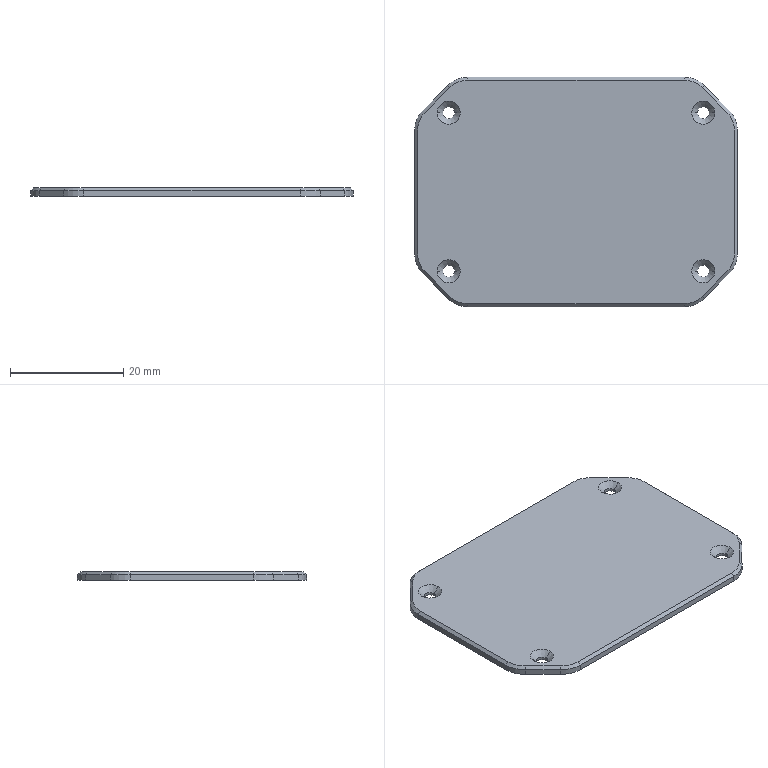NC program | NX | posted with a generic post | part box 57 x 40.5 x 1.5 mm
Lines 2968 to 4443 of 7802:
(PLANAR_PROFILE_COPY_3_COPY , TOOL : D4)
N5796 T01 M6
N5798 G54
N5800 G17 G0 G90 X-183.9 Y91.609 S6500 M3
N5802 G43 Z20. H1
N5804 Z0.1
N5806 G94 G1 Y68.668 Z0.06 F1200.
N5808 X-184.173 Y67.266 Z0.057
N5810 X-184.719 Y65.947 Z0.055
N5812 X-185.518 Y64.763 Z0.052
N5814 X-190.763 Y59.518 Z0.04
N5816 X-191.947 Y58.719 Z0.037
N5818 X-193.266 Y58.173 Z0.035
N5820 X-194.668 Y57.9 Z0.032
N5822 X-234.332 Z-0.037
N5824 X-235.734 Y58.173 Z-0.04
N5826 X-237.053 Y58.719 Z-0.042
N5828 X-238.237 Y59.518 Z-0.045
N5830 X-243.482 Y64.763 Z-0.058
N5832 X-244.281 Y65.947 Z-0.06
N5834 X-244.827 Y67.266 Z-0.063
N5836 X-245.1 Y68.668 Z-0.065
N5838 Y91.832 Z-0.106
N5840 X-244.827 Y93.234 Z-0.108
N5842 X-244.281 Y94.553 Z-0.11
N5844 X-243.482 Y95.737 Z-0.113
N5846 X-238.237 Y100.982 Z-0.126
N5848 X-237.053 Y101.781 Z-0.128
N5850 X-235.734 Y102.327 Z-0.131
N5852 X-234.332 Y102.6 Z-0.133
N5854 X-194.668 Z-0.203
N5856 X-193.266 Y102.327 Z-0.205
N5858 X-191.947 Y101.781 Z-0.208
N5860 X-190.763 Y100.982 Z-0.21
N5862 X-185.518 Y95.737 Z-0.223
N5864 X-184.719 Y94.553 Z-0.226
N5866 X-184.173 Y93.234 Z-0.228
N5868 X-183.9 Y91.832 Z-0.231
N5870 Y68.668 Z-0.271
N5872 X-184.173 Y67.266 Z-0.273
N5874 X-184.719 Y65.947 Z-0.276
N5876 X-185.518 Y64.763 Z-0.278
N5878 X-190.763 Y59.518 Z-0.291
N5880 X-191.947 Y58.719 Z-0.294
N5882 X-193.266 Y58.173 Z-0.296
N5884 X-194.668 Y57.9 Z-0.299
N5886 X-195.321 Z-0.3
N5888 X-233.679 F2000.
N5890 G2 X-238.699 Y59.98 R7.1
N5892 G1 X-243.02 Y64.301
N5894 G2 X-245.1 Y69.321 R7.1
N5896 G1 Y91.179
N5898 G2 X-243.02 Y96.199 R7.1
N5900 G1 X-238.699 Y100.52
N5902 G2 X-233.679 Y102.6 R7.1
N5904 G1 X-195.321
N5906 G2 X-190.301 Y100.52 R7.1
N5908 G1 X-185.98 Y96.199
N5910 G2 X-183.9 Y91.179 R7.1
N5912 G1 Y69.321
N5914 G2 X-185.98 Y64.301 R7.1
N5916 G1 X-190.301 Y59.98
N5918 G2 X-195.321 Y57.9 R7.1
N5920 G1 Z-0.2
N5922 G0 Z20.
N5924 X-183.9 Y91.609
N5926 Z-0.2
N5928 G1 Y68.668 Z-0.24 F1200.
N5930 X-184.173 Y67.266 Z-0.243
N5932 X-184.719 Y65.947 Z-0.245
N5934 X-185.518 Y64.763 Z-0.248
N5936 X-190.763 Y59.518 Z-0.26
N5938 X-191.947 Y58.719 Z-0.263
N5940 X-193.266 Y58.173 Z-0.265
N5942 X-194.668 Y57.9 Z-0.268
N5944 X-234.332 Z-0.337
N5946 X-235.734 Y58.173 Z-0.34
N5948 X-237.053 Y58.719 Z-0.342
N5950 X-238.237 Y59.518 Z-0.345
N5952 X-243.482 Y64.763 Z-0.358
N5954 X-244.281 Y65.947 Z-0.36
N5956 X-244.827 Y67.266 Z-0.363
N5958 X-245.1 Y68.668 Z-0.365
N5960 Y91.832 Z-0.406
N5962 X-244.827 Y93.234 Z-0.408
N5964 X-244.281 Y94.553 Z-0.41
N5966 X-243.482 Y95.737 Z-0.413
N5968 X-238.237 Y100.982 Z-0.426
N5970 X-237.053 Y101.781 Z-0.428
N5972 X-235.734 Y102.327 Z-0.431
N5974 X-234.332 Y102.6 Z-0.433
N5976 X-194.668 Z-0.503
N5978 X-193.266 Y102.327 Z-0.505
N5980 X-191.947 Y101.781 Z-0.508
N5982 X-190.763 Y100.982 Z-0.51
N5984 X-185.518 Y95.737 Z-0.523
N5986 X-184.719 Y94.553 Z-0.526
N5988 X-184.173 Y93.234 Z-0.528
N5990 X-183.9 Y91.832 Z-0.531
N5992 Y68.668 Z-0.571
N5994 X-184.173 Y67.266 Z-0.573
N5996 X-184.719 Y65.947 Z-0.576
N5998 X-185.518 Y64.763 Z-0.578
N6000 X-190.763 Y59.518 Z-0.591
N6002 X-191.947 Y58.719 Z-0.594
N6004 X-193.266 Y58.173 Z-0.596
N6006 X-194.668 Y57.9 Z-0.599
N6008 X-195.321 Z-0.6
N6010 X-233.679 F2000.
N6012 G2 X-238.699 Y59.98 R7.1
N6014 G1 X-243.02 Y64.301
N6016 G2 X-245.1 Y69.321 R7.1
N6018 G1 Y91.179
N6020 G2 X-243.02 Y96.199 R7.1
N6022 G1 X-238.699 Y100.52
N6024 G2 X-233.679 Y102.6 R7.1
N6026 G1 X-195.321
N6028 G2 X-190.301 Y100.52 R7.1
N6030 G1 X-185.98 Y96.199
N6032 G2 X-183.9 Y91.179 R7.1
N6034 G1 Y69.321
N6036 G2 X-185.98 Y64.301 R7.1
N6038 G1 X-190.301 Y59.98
N6040 G2 X-195.321 Y57.9 R7.1
N6042 G1 Z-0.5
N6044 G0 Z20.
N6046 X-183.9 Y91.609
N6048 Z-0.5
N6050 G1 Y68.668 Z-0.54 F1200.
N6052 X-184.173 Y67.266 Z-0.543
N6054 X-184.719 Y65.947 Z-0.545
N6056 X-185.518 Y64.763 Z-0.548
N6058 X-190.763 Y59.518 Z-0.56
N6060 X-191.947 Y58.719 Z-0.563
N6062 X-193.266 Y58.173 Z-0.565
N6064 X-194.668 Y57.9 Z-0.568
N6066 X-234.332 Z-0.637
N6068 X-235.734 Y58.173 Z-0.64
N6070 X-237.053 Y58.719 Z-0.642
N6072 X-238.237 Y59.518 Z-0.645
N6074 X-243.482 Y64.763 Z-0.658
N6076 X-244.281 Y65.947 Z-0.66
N6078 X-244.827 Y67.266 Z-0.663
N6080 X-245.1 Y68.668 Z-0.665
N6082 Y91.832 Z-0.706
N6084 X-244.827 Y93.234 Z-0.708
N6086 X-244.281 Y94.553 Z-0.71
N6088 X-243.482 Y95.737 Z-0.713
N6090 X-238.237 Y100.982 Z-0.726
N6092 X-237.053 Y101.781 Z-0.728
N6094 X-235.734 Y102.327 Z-0.731
N6096 X-234.332 Y102.6 Z-0.733
N6098 X-194.668 Z-0.803
N6100 X-193.266 Y102.327 Z-0.805
N6102 X-191.947 Y101.781 Z-0.808
N6104 X-190.763 Y100.982 Z-0.81
N6106 X-185.518 Y95.737 Z-0.823
N6108 X-184.719 Y94.553 Z-0.826
N6110 X-184.173 Y93.234 Z-0.828
N6112 X-183.9 Y91.832 Z-0.831
N6114 Y68.668 Z-0.871
N6116 X-184.173 Y67.266 Z-0.873
N6118 X-184.719 Y65.947 Z-0.876
N6120 X-185.518 Y64.763 Z-0.878
N6122 X-190.763 Y59.518 Z-0.891
N6124 X-191.947 Y58.719 Z-0.894
N6126 X-193.266 Y58.173 Z-0.896
N6128 X-194.668 Y57.9 Z-0.899
N6130 X-195.321 Z-0.9
N6132 X-233.679 F2000.
N6134 G2 X-238.699 Y59.98 R7.1
N6136 G1 X-243.02 Y64.301
N6138 G2 X-245.1 Y69.321 R7.1
N6140 G1 Y91.179
N6142 G2 X-243.02 Y96.199 R7.1
N6144 G1 X-238.699 Y100.52
N6146 G2 X-233.679 Y102.6 R7.1
N6148 G1 X-195.321
N6150 G2 X-190.301 Y100.52 R7.1
N6152 G1 X-185.98 Y96.199
N6154 G2 X-183.9 Y91.179 R7.1
N6156 G1 Y69.321
N6158 G2 X-185.98 Y64.301 R7.1
N6160 G1 X-190.301 Y59.98
N6162 G2 X-195.321 Y57.9 R7.1
N6164 G1 Z-0.8
N6166 G0 Z20.
N6168 X-183.9 Y91.609
N6170 Z-0.8
N6172 G1 Y68.668 Z-0.84 F1200.
N6174 X-184.173 Y67.266 Z-0.843
N6176 X-184.719 Y65.947 Z-0.845
N6178 X-185.518 Y64.763 Z-0.848
N6180 X-190.763 Y59.518 Z-0.86
N6182 X-191.947 Y58.719 Z-0.863
N6184 X-193.266 Y58.173 Z-0.865
N6186 X-194.668 Y57.9 Z-0.868
N6188 X-234.332 Z-0.937
N6190 X-235.734 Y58.173 Z-0.94
N6192 X-237.053 Y58.719 Z-0.942
N6194 X-238.237 Y59.518 Z-0.945
N6196 X-243.482 Y64.763 Z-0.958
N6198 X-244.281 Y65.947 Z-0.96
N6200 X-244.827 Y67.266 Z-0.963
N6202 X-245.1 Y68.668 Z-0.965
N6204 Y91.832 Z-1.006
N6206 X-244.827 Y93.234 Z-1.008
N6208 X-244.281 Y94.553 Z-1.01
N6210 X-243.482 Y95.737 Z-1.013
N6212 X-238.237 Y100.982 Z-1.026
N6214 X-237.053 Y101.781 Z-1.028
N6216 X-235.734 Y102.327 Z-1.031
N6218 X-234.332 Y102.6 Z-1.033
N6220 X-194.668 Z-1.103
N6222 X-193.266 Y102.327 Z-1.105
N6224 X-191.947 Y101.781 Z-1.108
N6226 X-190.763 Y100.982 Z-1.11
N6228 X-185.518 Y95.737 Z-1.123
N6230 X-184.719 Y94.553 Z-1.126
N6232 X-184.173 Y93.234 Z-1.128
N6234 X-183.9 Y91.832 Z-1.131
N6236 Y68.668 Z-1.171
N6238 X-184.173 Y67.266 Z-1.173
N6240 X-184.719 Y65.947 Z-1.176
N6242 X-185.518 Y64.763 Z-1.178
N6244 X-190.763 Y59.518 Z-1.191
N6246 X-191.947 Y58.719 Z-1.194
N6248 X-193.266 Y58.173 Z-1.196
N6250 X-194.668 Y57.9 Z-1.199
N6252 X-195.321 Z-1.2
N6254 X-233.679 F2000.
N6256 G2 X-238.699 Y59.98 R7.1
N6258 G1 X-243.02 Y64.301
N6260 G2 X-245.1 Y69.321 R7.1
N6262 G1 Y91.179
N6264 G2 X-243.02 Y96.199 R7.1
N6266 G1 X-238.699 Y100.52
N6268 G2 X-233.679 Y102.6 R7.1
N6270 G1 X-195.321
N6272 G2 X-190.301 Y100.52 R7.1
N6274 G1 X-185.98 Y96.199
N6276 G2 X-183.9 Y91.179 R7.1
N6278 G1 Y69.321
N6280 G2 X-185.98 Y64.301 R7.1
N6282 G1 X-190.301 Y59.98
N6284 G2 X-195.321 Y57.9 R7.1
N6286 G1 Z-1.1
N6288 G0 Z20.
N6290 X-183.9 Y91.609
N6292 Z-1.1
N6294 G1 Y68.668 Z-1.14 F1200.
N6296 X-184.173 Y67.266 Z-1.143
N6298 X-184.719 Y65.947 Z-1.145
N6300 X-185.518 Y64.763 Z-1.148
N6302 X-190.763 Y59.518 Z-1.16
N6304 X-191.947 Y58.719 Z-1.163
N6306 X-193.266 Y58.173 Z-1.165
N6308 X-194.668 Y57.9 Z-1.168
N6310 X-234.332 Z-1.237
N6312 X-235.734 Y58.173 Z-1.24
N6314 X-237.053 Y58.719 Z-1.242
N6316 X-238.237 Y59.518 Z-1.245
N6318 X-243.482 Y64.763 Z-1.258
N6320 X-244.281 Y65.947 Z-1.26
N6322 X-244.827 Y67.266 Z-1.263
N6324 X-245.1 Y68.668 Z-1.265
N6326 Y91.832 Z-1.306
N6328 X-244.827 Y93.234 Z-1.308
N6330 X-244.281 Y94.553 Z-1.31
N6332 X-243.482 Y95.737 Z-1.313
N6334 X-238.237 Y100.982 Z-1.326
N6336 X-237.053 Y101.781 Z-1.328
N6338 X-235.734 Y102.327 Z-1.331
N6340 X-234.332 Y102.6 Z-1.333
N6342 X-194.668 Z-1.403
N6344 X-193.266 Y102.327 Z-1.405
N6346 X-191.947 Y101.781 Z-1.408
N6348 X-190.763 Y100.982 Z-1.41
N6350 X-185.518 Y95.737 Z-1.423
N6352 X-184.719 Y94.553 Z-1.426
N6354 X-184.173 Y93.234 Z-1.428
N6356 X-183.9 Y91.832 Z-1.431
N6358 Y68.668 Z-1.471
N6360 X-184.173 Y67.266 Z-1.473
N6362 X-184.719 Y65.947 Z-1.476
N6364 X-185.518 Y64.763 Z-1.478
N6366 X-190.763 Y59.518 Z-1.491
N6368 X-191.947 Y58.719 Z-1.494
N6370 X-193.266 Y58.173 Z-1.496
N6372 X-194.668 Y57.9 Z-1.499
N6374 X-195.321 Z-1.5
N6376 X-233.679 F2000.
N6378 G2 X-238.699 Y59.98 R7.1
N6380 G1 X-243.02 Y64.301
N6382 G2 X-245.1 Y69.321 R7.1
N6384 G1 Y91.179
N6386 G2 X-243.02 Y96.199 R7.1
N6388 G1 X-238.699 Y100.52
N6390 G2 X-233.679 Y102.6 R7.1
N6392 G1 X-195.321
N6394 G2 X-190.301 Y100.52 R7.1
N6396 G1 X-185.98 Y96.199
N6398 G2 X-183.9 Y91.179 R7.1
N6400 G1 Y69.321
N6402 G2 X-185.98 Y64.301 R7.1
N6404 G1 X-190.301 Y59.98
N6406 G2 X-195.321 Y57.9 R7.1
N6408 G1 Z-1.4
N6410 G0 Z20.
(PLANAR_PROFILE_COPY_COPY_3_COPY , TOOL : D4)
N6412 X-195.221
N6414 Z1.5
N6416 G1 Z-1.5 F800.
N6418 X-195.232 Y57.952
N6420 X-195.27 Y57.989
N6422 X-195.321 Y58.
N6424 X-233.679
N6426 G2 X-238.629 Y60.05 R7.
N6428 G1 X-242.95 Y64.371
N6430 G2 X-245. Y69.321 R7.
N6432 G1 Y91.179
N6434 G2 X-242.95 Y96.129 R7.
N6436 G1 X-238.629 Y100.45
N6438 G2 X-233.679 Y102.5 R7.
N6440 G1 X-195.321
N6442 G2 X-190.371 Y100.45 R7.
N6444 G1 X-186.05 Y96.129
N6446 G2 X-184. Y91.179 R7.
N6448 G1 Y69.321
N6450 G2 X-186.05 Y64.371 R7.
N6452 G1 X-190.371 Y60.05
N6454 G2 X-195.321 Y58. R7.
N6456 G1 X-195.373 Y57.989
N6458 X-195.41 Y57.952
N6460 X-195.421 Y57.9
N6462 Z1.5
N6464 G0 Z20.
N6466 M5
(PLANAR_PROFILE_COPY_COPY_COPY_2_COPY , TOOL : D3倒角)
N6468 T02 M6
N6470 G54
N6472 G17 G0 G90 X-193.321 Y57.4 S4500 M3
N6474 G43 Z20. H2
N6476 Z2.
N6478 G94 G1 Z-1. F800.
N6480 G3 X-195.321 Y59.4 R2.
N6482 G1 X-233.679
N6484 G2 X-237.639 Y61.04 R5.6
N6486 G1 X-241.96 Y65.361
N6488 G2 X-243.6 Y69.321 R5.6
N6490 G1 Y91.179
N6492 G2 X-241.96 Y95.139 R5.6
N6494 G1 X-237.639 Y99.46
N6496 G2 X-233.679 Y101.1 R5.6
N6498 G1 X-195.321
N6500 G2 X-191.361 Y99.46 R5.6
N6502 G1 X-187.04 Y95.139
N6504 G2 X-185.4 Y91.179 R5.6
N6506 G1 Y69.321
N6508 G2 X-187.04 Y65.361 R5.6
N6510 G1 X-191.361 Y61.04
N6512 G2 X-195.321 Y59.4 R5.6
N6514 G3 X-197.321 Y57.4 R2.
N6516 G1 Z2.
N6518 G0 Z20.
N6520 M5
(PLANAR_PROFILE_COPY_4_COPY , TOOL : D4)
N6522 T01 M6
N6524 G54
N6526 G17 G0 G90 X-245.9 Y91.609 S6500 M3
N6528 G43 Z20. H1
N6530 Z0.1
N6532 G94 G1 Y68.668 Z0.06 F1200.
N6534 X-246.173 Y67.266 Z0.057
N6536 X-246.719 Y65.947 Z0.055
N6538 X-247.518 Y64.763 Z0.052
N6540 X-252.763 Y59.518 Z0.04
N6542 X-253.947 Y58.719 Z0.037
N6544 X-255.266 Y58.173 Z0.035
N6546 X-256.668 Y57.9 Z0.032
N6548 X-296.332 Z-0.037
N6550 X-297.734 Y58.173 Z-0.04
N6552 X-299.053 Y58.719 Z-0.042
N6554 X-300.237 Y59.518 Z-0.045
N6556 X-305.482 Y64.763 Z-0.058
N6558 X-306.281 Y65.947 Z-0.06
N6560 X-306.827 Y67.266 Z-0.063
N6562 X-307.1 Y68.668 Z-0.065
N6564 Y91.832 Z-0.106
N6566 X-306.827 Y93.234 Z-0.108
N6568 X-306.281 Y94.553 Z-0.11
N6570 X-305.482 Y95.737 Z-0.113
N6572 X-300.237 Y100.982 Z-0.126
N6574 X-299.053 Y101.781 Z-0.128
N6576 X-297.734 Y102.327 Z-0.131
N6578 X-296.332 Y102.6 Z-0.133
N6580 X-256.668 Z-0.203
N6582 X-255.266 Y102.327 Z-0.205
N6584 X-253.947 Y101.781 Z-0.208
N6586 X-252.763 Y100.982 Z-0.21
N6588 X-247.518 Y95.737 Z-0.223
N6590 X-246.719 Y94.553 Z-0.226
N6592 X-246.173 Y93.234 Z-0.228
N6594 X-245.9 Y91.832 Z-0.231
N6596 Y68.668 Z-0.271
N6598 X-246.173 Y67.266 Z-0.273
N6600 X-246.719 Y65.947 Z-0.276
N6602 X-247.518 Y64.763 Z-0.278
N6604 X-252.763 Y59.518 Z-0.291
N6606 X-253.947 Y58.719 Z-0.294
N6608 X-255.266 Y58.173 Z-0.296
N6610 X-256.668 Y57.9 Z-0.299
N6612 X-257.321 Z-0.3
N6614 X-295.679 F2000.
N6616 G2 X-300.699 Y59.98 R7.1
N6618 G1 X-305.02 Y64.301
N6620 G2 X-307.1 Y69.321 R7.1
N6622 G1 Y91.179
N6624 G2 X-305.02 Y96.199 R7.1
N6626 G1 X-300.699 Y100.52
N6628 G2 X-295.679 Y102.6 R7.1
N6630 G1 X-257.321
N6632 G2 X-252.301 Y100.52 R7.1
N6634 G1 X-247.98 Y96.199
N6636 G2 X-245.9 Y91.179 R7.1
N6638 G1 Y69.321
N6640 G2 X-247.98 Y64.301 R7.1
N6642 G1 X-252.301 Y59.98
N6644 G2 X-257.321 Y57.9 R7.1
N6646 G1 Z-0.2
N6648 G0 Z20.
N6650 X-245.9 Y91.609
N6652 Z-0.2
N6654 G1 Y68.668 Z-0.24 F1200.
N6656 X-246.173 Y67.266 Z-0.243
N6658 X-246.719 Y65.947 Z-0.245
N6660 X-247.518 Y64.763 Z-0.248
N6662 X-252.763 Y59.518 Z-0.26
N6664 X-253.947 Y58.719 Z-0.263
N6666 X-255.266 Y58.173 Z-0.265
N6668 X-256.668 Y57.9 Z-0.268
N6670 X-296.332 Z-0.337
N6672 X-297.734 Y58.173 Z-0.34
N6674 X-299.053 Y58.719 Z-0.342
N6676 X-300.237 Y59.518 Z-0.345
N6678 X-305.482 Y64.763 Z-0.358
N6680 X-306.281 Y65.947 Z-0.36
N6682 X-306.827 Y67.266 Z-0.363
N6684 X-307.1 Y68.668 Z-0.365
N6686 Y91.832 Z-0.406
N6688 X-306.827 Y93.234 Z-0.408
N6690 X-306.281 Y94.553 Z-0.41
N6692 X-305.482 Y95.737 Z-0.413
N6694 X-300.237 Y100.982 Z-0.426
N6696 X-299.053 Y101.781 Z-0.428
N6698 X-297.734 Y102.327 Z-0.431
N6700 X-296.332 Y102.6 Z-0.433
N6702 X-256.668 Z-0.503
N6704 X-255.266 Y102.327 Z-0.505
N6706 X-253.947 Y101.781 Z-0.508
N6708 X-252.763 Y100.982 Z-0.51
N6710 X-247.518 Y95.737 Z-0.523
N6712 X-246.719 Y94.553 Z-0.526
N6714 X-246.173 Y93.234 Z-0.528
N6716 X-245.9 Y91.832 Z-0.531
N6718 Y68.668 Z-0.571
N6720 X-246.173 Y67.266 Z-0.573
N6722 X-246.719 Y65.947 Z-0.576
N6724 X-247.518 Y64.763 Z-0.578
N6726 X-252.763 Y59.518 Z-0.591
N6728 X-253.947 Y58.719 Z-0.594
N6730 X-255.266 Y58.173 Z-0.596
N6732 X-256.668 Y57.9 Z-0.599
N6734 X-257.321 Z-0.6
N6736 X-295.679 F2000.
N6738 G2 X-300.699 Y59.98 R7.1
N6740 G1 X-305.02 Y64.301
N6742 G2 X-307.1 Y69.321 R7.1
N6744 G1 Y91.179
N6746 G2 X-305.02 Y96.199 R7.1
N6748 G1 X-300.699 Y100.52
N6750 G2 X-295.679 Y102.6 R7.1
N6752 G1 X-257.321
N6754 G2 X-252.301 Y100.52 R7.1
N6756 G1 X-247.98 Y96.199
N6758 G2 X-245.9 Y91.179 R7.1
N6760 G1 Y69.321
N6762 G2 X-247.98 Y64.301 R7.1
N6764 G1 X-252.301 Y59.98
N6766 G2 X-257.321 Y57.9 R7.1
N6768 G1 Z-0.5
N6770 G0 Z20.
N6772 X-245.9 Y91.609
N6774 Z-0.5
N6776 G1 Y68.668 Z-0.54 F1200.
N6778 X-246.173 Y67.266 Z-0.543
N6780 X-246.719 Y65.947 Z-0.545
N6782 X-247.518 Y64.763 Z-0.548
N6784 X-252.763 Y59.518 Z-0.56
N6786 X-253.947 Y58.719 Z-0.563
N6788 X-255.266 Y58.173 Z-0.565
N6790 X-256.668 Y57.9 Z-0.568
N6792 X-296.332 Z-0.637
N6794 X-297.734 Y58.173 Z-0.64
N6796 X-299.053 Y58.719 Z-0.642
N6798 X-300.237 Y59.518 Z-0.645
N6800 X-305.482 Y64.763 Z-0.658
N6802 X-306.281 Y65.947 Z-0.66
N6804 X-306.827 Y67.266 Z-0.663
N6806 X-307.1 Y68.668 Z-0.665
N6808 Y91.832 Z-0.706
N6810 X-306.827 Y93.234 Z-0.708
N6812 X-306.281 Y94.553 Z-0.71
N6814 X-305.482 Y95.737 Z-0.713
N6816 X-300.237 Y100.982 Z-0.726
N6818 X-299.053 Y101.781 Z-0.728
N6820 X-297.734 Y102.327 Z-0.731
N6822 X-296.332 Y102.6 Z-0.733
N6824 X-256.668 Z-0.803
N6826 X-255.266 Y102.327 Z-0.805
N6828 X-253.947 Y101.781 Z-0.808
N6830 X-252.763 Y100.982 Z-0.81
N6832 X-247.518 Y95.737 Z-0.823
N6834 X-246.719 Y94.553 Z-0.826
N6836 X-246.173 Y93.234 Z-0.828
N6838 X-245.9 Y91.832 Z-0.831
N6840 Y68.668 Z-0.871
N6842 X-246.173 Y67.266 Z-0.873
N6844 X-246.719 Y65.947 Z-0.876
N6846 X-247.518 Y64.763 Z-0.878
N6848 X-252.763 Y59.518 Z-0.891
N6850 X-253.947 Y58.719 Z-0.894
N6852 X-255.266 Y58.173 Z-0.896
N6854 X-256.668 Y57.9 Z-0.899
N6856 X-257.321 Z-0.9
N6858 X-295.679 F2000.
N6860 G2 X-300.699 Y59.98 R7.1
N6862 G1 X-305.02 Y64.301
N6864 G2 X-307.1 Y69.321 R7.1
N6866 G1 Y91.179
N6868 G2 X-305.02 Y96.199 R7.1
N6870 G1 X-300.699 Y100.52
N6872 G2 X-295.679 Y102.6 R7.1
N6874 G1 X-257.321
N6876 G2 X-252.301 Y100.52 R7.1
N6878 G1 X-247.98 Y96.199
N6880 G2 X-245.9 Y91.179 R7.1
N6882 G1 Y69.321
N6884 G2 X-247.98 Y64.301 R7.1
N6886 G1 X-252.301 Y59.98
N6888 G2 X-257.321 Y57.9 R7.1
N6890 G1 Z-0.8
N6892 G0 Z20.
N6894 X-245.9 Y91.609
N6896 Z-0.8
N6898 G1 Y68.668 Z-0.84 F1200.
N6900 X-246.173 Y67.266 Z-0.843
N6902 X-246.719 Y65.947 Z-0.845
N6904 X-247.518 Y64.763 Z-0.848
N6906 X-252.763 Y59.518 Z-0.86
N6908 X-253.947 Y58.719 Z-0.863
N6910 X-255.266 Y58.173 Z-0.865
N6912 X-256.668 Y57.9 Z-0.868
N6914 X-296.332 Z-0.937
N6916 X-297.734 Y58.173 Z-0.94
N6918 X-299.053 Y58.719 Z-0.942
N6920 X-300.237 Y59.518 Z-0.945
N6922 X-305.482 Y64.763 Z-0.958
N6924 X-306.281 Y65.947 Z-0.96
N6926 X-306.827 Y67.266 Z-0.963
N6928 X-307.1 Y68.668 Z-0.965
N6930 Y91.832 Z-1.006
N6932 X-306.827 Y93.234 Z-1.008
N6934 X-306.281 Y94.553 Z-1.01
N6936 X-305.482 Y95.737 Z-1.013
N6938 X-300.237 Y100.982 Z-1.026
N6940 X-299.053 Y101.781 Z-1.028
N6942 X-297.734 Y102.327 Z-1.031
N6944 X-296.332 Y102.6 Z-1.033
N6946 X-256.668 Z-1.103
N6948 X-255.266 Y102.327 Z-1.105
N6950 X-253.947 Y101.781 Z-1.108
N6952 X-252.763 Y100.982 Z-1.11
N6954 X-247.518 Y95.737 Z-1.123
N6956 X-246.719 Y94.553 Z-1.126
N6958 X-246.173 Y93.234 Z-1.128
N6960 X-245.9 Y91.832 Z-1.131
N6962 Y68.668 Z-1.171
N6964 X-246.173 Y67.266 Z-1.173
N6966 X-246.719 Y65.947 Z-1.176
N6968 X-247.518 Y64.763 Z-1.178
N6970 X-252.763 Y59.518 Z-1.191
N6972 X-253.947 Y58.719 Z-1.194
N6974 X-255.266 Y58.173 Z-1.196
N6976 X-256.668 Y57.9 Z-1.199
N6978 X-257.321 Z-1.2
N6980 X-295.679 F2000.
N6982 G2 X-300.699 Y59.98 R7.1
N6984 G1 X-305.02 Y64.301
N6986 G2 X-307.1 Y69.321 R7.1
N6988 G1 Y91.179
N6990 G2 X-305.02 Y96.199 R7.1
N6992 G1 X-300.699 Y100.52
N6994 G2 X-295.679 Y102.6 R7.1
N6996 G1 X-257.321
N6998 G2 X-252.301 Y100.52 R7.1
N7000 G1 X-247.98 Y96.199
N7002 G2 X-245.9 Y91.179 R7.1
N7004 G1 Y69.321
N7006 G2 X-247.98 Y64.301 R7.1
N7008 G1 X-252.301 Y59.98
N7010 G2 X-257.321 Y57.9 R7.1
N7012 G1 Z-1.1
N7014 G0 Z20.
N7016 X-302.406 Y61.686
N7018 Z-1.1
N7020 G1 X-305.482 Y64.763 Z-1.108 F1200.
N7022 X-306.281 Y65.947 Z-1.11
N7024 X-306.827 Y67.266 Z-1.113
N7026 X-307.1 Y68.668 Z-1.115
N7028 Y91.832 Z-1.156
N7030 X-306.827 Y93.234 Z-1.158
N7032 X-306.281 Y94.553 Z-1.16
N7034 X-305.482 Y95.737 Z-1.163
N7036 X-300.237 Y100.982 Z-1.176
N7038 X-299.053 Y101.781 Z-1.178
N7040 X-297.734 Y102.327 Z-1.181
N7042 X-296.332 Y102.6 Z-1.183
N7044 X-256.668 Z-1.253
N7046 X-255.266 Y102.327 Z-1.255
N7048 X-253.947 Y101.781 Z-1.258
N7050 X-252.763 Y100.982 Z-1.26
N7052 X-247.518 Y95.737 Z-1.273
N7054 X-246.719 Y94.553 Z-1.276
N7056 X-246.173 Y93.234 Z-1.278
N7058 X-245.9 Y91.832 Z-1.281
N7060 Y68.668 Z-1.321
N7062 X-246.173 Y67.266 Z-1.323
N7064 X-246.719 Y65.947 Z-1.326
N7066 X-247.518 Y64.763 Z-1.328
N7068 X-252.763 Y59.518 Z-1.341
N7070 X-253.947 Y58.719 Z-1.344
N7072 X-255.266 Y58.173 Z-1.346
N7074 X-256.668 Y57.9 Z-1.349
N7076 X-257.321 Z-1.35
N7078 X-295.679 F2000.
N7080 G2 X-300.699 Y59.98 R7.1
N7082 G1 X-305.02 Y64.301
N7084 G2 X-307.1 Y69.321 R7.1
N7086 G1 Y91.179
N7088 G2 X-305.02 Y96.199 R7.1
N7090 G1 X-300.699 Y100.52
N7092 G2 X-295.679 Y102.6 R7.1
N7094 G1 X-257.321
N7096 G2 X-252.301 Y100.52 R7.1
N7098 G1 X-247.98 Y96.199
N7100 G2 X-245.9 Y91.179 R7.1
N7102 G1 Y69.321
N7104 G2 X-247.98 Y64.301 R7.1
N7106 G1 X-252.301 Y59.98
N7108 G2 X-257.321 Y57.9 R7.1
N7110 G1 Z-1.25
N7112 G0 Z20.
(PLANAR_PROFILE_COPY_COPY_4_COPY , TOOL : D4)
N7114 X-257.221
N7116 Z1.65
N7118 G1 Z-1.35 F800.
N7120 X-257.232 Y57.952
N7122 X-257.27 Y57.989
N7124 X-257.321 Y58.
N7126 X-295.679
N7128 G2 X-300.629 Y60.05 R7.
N7130 G1 X-304.95 Y64.371
N7132 G2 X-307. Y69.321 R7.
N7134 G1 Y91.179
N7136 G2 X-304.95 Y96.129 R7.
N7138 G1 X-300.629 Y100.45
N7140 G2 X-295.679 Y102.5 R7.
N7142 G1 X-257.321
N7144 G2 X-252.371 Y100.45 R7.
N7146 G1 X-248.05 Y96.129
N7148 G2 X-246. Y91.179 R7.
N7150 G1 Y69.321
N7152 G2 X-248.05 Y64.371 R7.
N7154 G1 X-252.371 Y60.05
N7156 G2 X-257.321 Y58. R7.
N7158 G1 X-257.373 Y57.989
N7160 X-257.41 Y57.952
N7162 X-257.421 Y57.9
N7164 Z1.65
N7166 G0 Z20.
N7168 M5
(PLANAR_PROFILE_COPY_COPY_COPY_3_COPY , TOOL : D3倒角)
N7170 T02 M6
N7172 G54
N7174 G17 G0 G90 X-255.321 Y57.4 S4500 M3
N7176 G43 Z20. H2
N7178 Z2.
N7180 G94 G1 Z-1. F800.
N7182 G3 X-257.321 Y59.4 R2.
N7184 G1 X-295.679
N7186 G2 X-299.639 Y61.04 R5.6
N7188 G1 X-303.96 Y65.361
N7190 G2 X-305.6 Y69.321 R5.6
N7192 G1 Y91.179
N7194 G2 X-303.96 Y95.139 R5.6
N7196 G1 X-299.639 Y99.46
N7198 G2 X-295.679 Y101.1 R5.6
N7200 G1 X-257.321
N7202 G2 X-253.361 Y99.46 R5.6
N7204 G1 X-249.04 Y95.139
N7206 G2 X-247.4 Y91.179 R5.6
N7208 G1 Y69.321
N7210 G2 X-249.04 Y65.361 R5.6
N7212 G1 X-253.361 Y61.04
N7214 G2 X-257.321 Y59.4 R5.6
N7216 G3 X-259.321 Y57.4 R2.
N7218 G1 Z2.
N7220 G0 Z20.
N7222 M5
(PLANAR_PROFILE_COPY_6 , TOOL : D4)
N7224 T01 M6
N7226 G54
N7228 G17 G0 G90 X2.1 Y151.609 S6500 M3
N7230 G43 Z20. H1
N7232 Z0.1
N7234 G94 G1 Y128.668 Z0.06 F1200.
N7236 X1.827 Y127.266 Z0.057
N7238 X1.281 Y125.947 Z0.055
N7240 X0.482 Y124.763 Z0.052
N7242 X-4.763 Y119.518 Z0.04
N7244 X-5.947 Y118.719 Z0.037
N7246 X-7.266 Y118.173 Z0.035
N7248 X-8.668 Y117.9 Z0.032
N7250 X-48.332 Z-0.037
N7252 X-49.734 Y118.173 Z-0.04
N7254 X-51.053 Y118.719 Z-0.042
N7256 X-52.237 Y119.518 Z-0.045
N7258 X-57.482 Y124.763 Z-0.058
N7260 X-58.281 Y125.947 Z-0.06
N7262 X-58.827 Y127.266 Z-0.063
N7264 X-59.1 Y128.668 Z-0.065
N7266 Y151.832 Z-0.106
N7268 X-58.827 Y153.234 Z-0.108
N7270 X-58.281 Y154.553 Z-0.11
N7272 X-57.482 Y155.737 Z-0.113
N7274 X-52.237 Y160.982 Z-0.126
N7276 X-51.053 Y161.781 Z-0.128
N7278 X-49.734 Y162.327 Z-0.131
N7280 X-48.332 Y162.6 Z-0.133
N7282 X-8.668 Z-0.203
N7284 X-7.266 Y162.327 Z-0.205
N7286 X-5.947 Y161.781 Z-0.208
N7288 X-4.763 Y160.982 Z-0.21
N7290 X0.482 Y155.737 Z-0.223
N7292 X1.281 Y154.553 Z-0.226
N7294 X1.827 Y153.234 Z-0.228
N7296 X2.1 Y151.832 Z-0.231
N7298 Y128.668 Z-0.271
N7300 X1.827 Y127.266 Z-0.273
N7302 X1.281 Y125.947 Z-0.276
N7304 X0.482 Y124.763 Z-0.278
N7306 X-4.763 Y119.518 Z-0.291
N7308 X-5.947 Y118.719 Z-0.294
N7310 X-7.266 Y118.173 Z-0.296
N7312 X-8.668 Y117.9 Z-0.299
N7314 X-9.321 Z-0.3
N7316 X-47.679 F2000.
N7318 G2 X-52.699 Y119.98 R7.1
N7320 G1 X-57.02 Y124.301
N7322 G2 X-59.1 Y129.321 R7.1
N7324 G1 Y151.179
N7326 G2 X-57.02 Y156.199 R7.1
N7328 G1 X-52.699 Y160.52
N7330 G2 X-47.679 Y162.6 R7.1
N7332 G1 X-9.321
N7334 G2 X-4.301 Y160.52 R7.1
N7336 G1 X0.02 Y156.199
N7338 G2 X2.1 Y151.179 R7.1
N7340 G1 Y129.321
N7342 G2 X0.02 Y124.301 R7.1
N7344 G1 X-4.301 Y119.98
N7346 G2 X-9.321 Y117.9 R7.1
N7348 G1 Z-0.2
N7350 G0 Z20.
N7352 X2.1 Y151.609
N7354 Z-0.2
N7356 G1 Y128.668 Z-0.24 F1200.
N7358 X1.827 Y127.266 Z-0.243
N7360 X1.281 Y125.947 Z-0.245
N7362 X0.482 Y124.763 Z-0.248
N7364 X-4.763 Y119.518 Z-0.26
N7366 X-5.947 Y118.719 Z-0.263
N7368 X-7.266 Y118.173 Z-0.265
N7370 X-8.668 Y117.9 Z-0.268
N7372 X-48.332 Z-0.337
N7374 X-49.734 Y118.173 Z-0.34
N7376 X-51.053 Y118.719 Z-0.342
N7378 X-52.237 Y119.518 Z-0.345
N7380 X-57.482 Y124.763 Z-0.358
N7382 X-58.281 Y125.947 Z-0.36
N7384 X-58.827 Y127.266 Z-0.363
N7386 X-59.1 Y128.668 Z-0.365
N7388 Y151.832 Z-0.406
N7390 X-58.827 Y153.234 Z-0.408
N7392 X-58.281 Y154.553 Z-0.41
N7394 X-57.482 Y155.737 Z-0.413
N7396 X-52.237 Y160.982 Z-0.426
N7398 X-51.053 Y161.781 Z-0.428
N7400 X-49.734 Y162.327 Z-0.431
N7402 X-48.332 Y162.6 Z-0.433
N7404 X-8.668 Z-0.503
N7406 X-7.266 Y162.327 Z-0.505
N7408 X-5.947 Y161.781 Z-0.508
N7410 X-4.763 Y160.982 Z-0.51
N7412 X0.482 Y155.737 Z-0.523
N7414 X1.281 Y154.553 Z-0.526
N7416 X1.827 Y153.234 Z-0.528
N7418 X2.1 Y151.832 Z-0.531
N7420 Y128.668 Z-0.571
N7422 X1.827 Y127.266 Z-0.573
N7424 X1.281 Y125.947 Z-0.576
N7426 X0.482 Y124.763 Z-0.578
N7428 X-4.763 Y119.518 Z-0.591
N7430 X-5.947 Y118.719 Z-0.594
N7432 X-7.266 Y118.173 Z-0.596
N7434 X-8.668 Y117.9 Z-0.599
N7436 X-9.321 Z-0.6
N7438 X-47.679 F2000.
N7440 G2 X-52.699 Y119.98 R7.1
N7442 G1 X-57.02 Y124.301
N7444 G2 X-59.1 Y129.321 R7.1
N7446 G1 Y151.179
N7448 G2 X-57.02 Y156.199 R7.1
N7450 G1 X-52.699 Y160.52
N7452 G2 X-47.679 Y162.6 R7.1
N7454 G1 X-9.321
N7456 G2 X-4.301 Y160.52 R7.1
N7458 G1 X0.02 Y156.199
N7460 G2 X2.1 Y151.179 R7.1
N7462 G1 Y129.321
N7464 G2 X0.02 Y124.301 R7.1
N7466 G1 X-4.301 Y119.98
N7468 G2 X-9.321 Y117.9 R7.1
N7470 G1 Z-0.5
N7472 G0 Z20.
N7474 X2.1 Y151.609
N7476 Z-0.5
N7478 G1 Y128.668 Z-0.54 F1200.
N7480 X1.827 Y127.266 Z-0.543
N7482 X1.281 Y125.947 Z-0.545
N7484 X0.482 Y124.763 Z-0.548
N7486 X-4.763 Y119.518 Z-0.56
N7488 X-5.947 Y118.719 Z-0.563
N7490 X-7.266 Y118.173 Z-0.565
N7492 X-8.668 Y117.9 Z-0.568
N7494 X-48.332 Z-0.637
N7496 X-49.734 Y118.173 Z-0.64
N7498 X-51.053 Y118.719 Z-0.642
N7500 X-52.237 Y119.518 Z-0.645
N7502 X-57.482 Y124.763 Z-0.658
N7504 X-58.281 Y125.947 Z-0.66
N7506 X-58.827 Y127.266 Z-0.663
N7508 X-59.1 Y128.668 Z-0.665
N7510 Y151.832 Z-0.706
N7512 X-58.827 Y153.234 Z-0.708
N7514 X-58.281 Y154.553 Z-0.71
N7516 X-57.482 Y155.737 Z-0.713
N7518 X-52.237 Y160.982 Z-0.726
N7520 X-51.053 Y161.781 Z-0.728
N7522 X-49.734 Y162.327 Z-0.731
N7524 X-48.332 Y162.6 Z-0.733
N7526 X-8.668 Z-0.803
N7528 X-7.266 Y162.327 Z-0.805
N7530 X-5.947 Y161.781 Z-0.808
N7532 X-4.763 Y160.982 Z-0.81
N7534 X0.482 Y155.737 Z-0.823
N7536 X1.281 Y154.553 Z-0.826
N7538 X1.827 Y153.234 Z-0.828
N7540 X2.1 Y151.832 Z-0.831
N7542 Y128.668 Z-0.871
N7544 X1.827 Y127.266 Z-0.873
N7546 X1.281 Y125.947 Z-0.876
N7548 X0.482 Y124.763 Z-0.878
N7550 X-4.763 Y119.518 Z-0.891
N7552 X-5.947 Y118.719 Z-0.894
N7554 X-7.266 Y118.173 Z-0.896
N7556 X-8.668 Y117.9 Z-0.899
N7558 X-9.321 Z-0.9
N7560 X-47.679 F2000.
N7562 G2 X-52.699 Y119.98 R7.1
N7564 G1 X-57.02 Y124.301
N7566 G2 X-59.1 Y129.321 R7.1
N7568 G1 Y151.179
N7570 G2 X-57.02 Y156.199 R7.1
N7572 G1 X-52.699 Y160.52
N7574 G2 X-47.679 Y162.6 R7.1
N7576 G1 X-9.321
N7578 G2 X-4.301 Y160.52 R7.1
N7580 G1 X0.02 Y156.199
N7582 G2 X2.1 Y151.179 R7.1
N7584 G1 Y129.321
N7586 G2 X0.02 Y124.301 R7.1
N7588 G1 X-4.301 Y119.98
N7590 G2 X-9.321 Y117.9 R7.1
N7592 G1 Z-0.8
N7594 G0 Z20.
N7596 X2.1 Y151.609
N7598 Z-0.8
N7600 G1 Y128.668 Z-0.84 F1200.
N7602 X1.827 Y127.266 Z-0.843
N7604 X1.281 Y125.947 Z-0.845
N7606 X0.482 Y124.763 Z-0.848
N7608 X-4.763 Y119.518 Z-0.86
N7610 X-5.947 Y118.719 Z-0.863
N7612 X-7.266 Y118.173 Z-0.865
N7614 X-8.668 Y117.9 Z-0.868
N7616 X-48.332 Z-0.937
N7618 X-49.734 Y118.173 Z-0.94
N7620 X-51.053 Y118.719 Z-0.942
N7622 X-52.237 Y119.518 Z-0.945
N7624 X-57.482 Y124.763 Z-0.958
N7626 X-58.281 Y125.947 Z-0.96
N7628 X-58.827 Y127.266 Z-0.963
N7630 X-59.1 Y128.668 Z-0.965
N7632 Y151.832 Z-1.006
N7634 X-58.827 Y153.234 Z-1.008
N7636 X-58.281 Y154.553 Z-1.01
N7638 X-57.482 Y155.737 Z-1.013
N7640 X-52.237 Y160.982 Z-1.026
N7642 X-51.053 Y161.781 Z-1.028
N7644 X-49.734 Y162.327 Z-1.031
N7646 X-48.332 Y162.6 Z-1.033
N7648 X-8.668 Z-1.103
N7650 X-7.266 Y162.327 Z-1.105
N7652 X-5.947 Y161.781 Z-1.108
N7654 X-4.763 Y160.982 Z-1.11
N7656 X0.482 Y155.737 Z-1.123
N7658 X1.281 Y154.553 Z-1.126
N7660 X1.827 Y153.234 Z-1.128
N7662 X2.1 Y151.832 Z-1.131
N7664 Y128.668 Z-1.171
N7666 X1.827 Y127.266 Z-1.173
N7668 X1.281 Y125.947 Z-1.176
N7670 X0.482 Y124.763 Z-1.178
N7672 X-4.763 Y119.518 Z-1.191
N7674 X-5.947 Y118.719 Z-1.194
N7676 X-7.266 Y118.173 Z-1.196
N7678 X-8.668 Y117.9 Z-1.199
N7680 X-9.321 Z-1.2
N7682 X-47.679 F2000.
N7684 G2 X-52.699 Y119.98 R7.1
N7686 G1 X-57.02 Y124.301
N7688 G2 X-59.1 Y129.321 R7.1
N7690 G1 Y151.179
N7692 G2 X-57.02 Y156.199 R7.1
N7694 G1 X-52.699 Y160.52
N7696 G2 X-47.679 Y162.6 R7.1
N7698 G1 X-9.321
N7700 G2 X-4.301 Y160.52 R7.1
N7702 G1 X0.02 Y156.199
N7704 G2 X2.1 Y151.179 R7.1
N7706 G1 Y129.321
N7708 G2 X0.02 Y124.301 R7.1
N7710 G1 X-4.301 Y119.98
N7712 G2 X-9.321 Y117.9 R7.1
N7714 G1 Z-1.1
N7716 G0 Z20.
N7718 X2.1 Y151.609
N7720 Z-1.1
N7722 G1 Y128.668 Z-1.14 F1200.
N7724 X1.827 Y127.266 Z-1.143
N7726 X1.281 Y125.947 Z-1.145
N7728 X0.482 Y124.763 Z-1.148
N7730 X-4.763 Y119.518 Z-1.16
N7732 X-5.947 Y118.719 Z-1.163
N7734 X-7.266 Y118.173 Z-1.165
N7736 X-8.668 Y117.9 Z-1.168
N7738 X-48.332 Z-1.237
N7740 X-49.734 Y118.173 Z-1.24
N7742 X-51.053 Y118.719 Z-1.242
N7744 X-52.237 Y119.518 Z-1.245
N7746 X-57.482 Y124.763 Z-1.258
N7748 X-58.281 Y125.947 Z-1.26
N7750 X-58.827 Y127.266 Z-1.263
N7752 X-59.1 Y128.668 Z-1.265
N7754 Y151.832 Z-1.306
N7756 X-58.827 Y153.234 Z-1.308
N7758 X-58.281 Y154.553 Z-1.31
N7760 X-57.482 Y155.737 Z-1.313
N7762 X-52.237 Y160.982 Z-1.326
N7764 X-51.053 Y161.781 Z-1.328
N7766 X-49.734 Y162.327 Z-1.331
N7768 X-48.332 Y162.6 Z-1.333
N7770 X-8.668 Z-1.403
N7772 X-7.266 Y162.327 Z-1.405
N7774 X-5.947 Y161.781 Z-1.408
N7776 X-4.763 Y160.982 Z-1.41
N7778 X0.482 Y155.737 Z-1.423
N7780 X1.281 Y154.553 Z-1.426
N7782 X1.827 Y153.234 Z-1.428
N7784 X2.1 Y151.832 Z-1.431
N7786 Y128.668 Z-1.471
N7788 X1.827 Y127.266 Z-1.473
N7790 X1.281 Y125.947 Z-1.476
N7792 X0.482 Y124.763 Z-1.478
N7794 X-4.763 Y119.518 Z-1.491
N7796 X-5.947 Y118.719 Z-1.494
N7798 X-7.266 Y118.173 Z-1.496
N7800 X-8.668 Y117.9 Z-1.499
N7802 X-9.321 Z-1.5
N7804 X-47.679 F2000.
N7806 G2 X-52.699 Y119.98 R7.1
N7808 G1 X-57.02 Y124.301
N7810 G2 X-59.1 Y129.321 R7.1
N7812 G1 Y151.179
N7814 G2 X-57.02 Y156.199 R7.1
N7816 G1 X-52.699 Y160.52
N7818 G2 X-47.679 Y162.6 R7.1
N7820 G1 X-9.321
N7822 G2 X-4.301 Y160.52 R7.1
N7824 G1 X0.02 Y156.199
N7826 G2 X2.1 Y151.179 R7.1
N7828 G1 Y129.321
N7830 G2 X0.02 Y124.301 R7.1
N7832 G1 X-4.301 Y119.98
N7834 G2 X-9.321 Y117.9 R7.1
N7836 G1 Z-1.4
N7838 G0 Z20.
(PLANAR_PROFILE_COPY_COPY_6 , TOOL : D4)
N7840 X-9.221
N7842 Z1.5
N7844 G1 Z-1.5 F800.
N7846 X-9.232 Y117.952
N7848 X-9.27 Y117.989
N7850 X-9.321 Y118.
N7852 X-47.679
N7854 G2 X-52.629 Y120.05 R7.
N7856 G1 X-56.95 Y124.371
N7858 G2 X-59. Y129.321 R7.
N7860 G1 Y151.179
N7862 G2 X-56.95 Y156.129 R7.
N7864 G1 X-52.629 Y160.45
N7866 G2 X-47.679 Y162.5 R7.
N7868 G1 X-9.321
N7870 G2 X-4.371 Y160.45 R7.
N7872 G1 X-0.05 Y156.129
N7874 G2 X2. Y151.179 R7.
N7876 G1 Y129.321
N7878 G2 X-0.05 Y124.371 R7.
N7880 G1 X-4.371 Y120.05
N7882 G2 X-9.321 Y118. R7.
N7884 G1 X-9.373 Y117.989
N7886 X-9.41 Y117.952
N7888 X-9.421 Y117.9
N7890 Z1.5
N7892 G0 Z20.
N7894 M5
(PLANAR_PROFILE_COPY_COPY_COPY_5 , TOOL : D3倒角)
N7896 T02 M6
N7898 G54
N7900 G17 G0 G90 X-7.321 Y117.4 S4500 M3
N7902 G43 Z20. H2
N7904 Z2.
N7906 G94 G1 Z-1. F800.
N7908 G3 X-9.321 Y119.4 R2.
N7910 G1 X-47.679
N7912 G2 X-51.639 Y121.04 R5.6
N7914 G1 X-55.96 Y125.361
N7916 G2 X-57.6 Y129.321 R5.6
N7918 G1 Y151.179
N7920 G2 X-55.96 Y155.139 R5.6
N7922 G1 X-51.639 Y159.46
N7924 G2 X-47.679 Y161.1 R5.6
N7926 G1 X-9.321
N7928 G2 X-5.361 Y159.46 R5.6
N7930 G1 X-1.04 Y155.139
N7932 G2 X0.6 Y151.179 R5.6
N7934 G1 Y129.321
N7936 G2 X-1.04 Y125.361 R5.6
N7938 G1 X-5.361 Y121.04
N7940 G2 X-9.321 Y119.4 R5.6
N7942 G3 X-11.321 Y117.4 R2.
N7944 G1 Z2.
N7946 G0 Z20.
N7948 M5
(PLANAR_PROFILE_COPY_1_COPY_1 , TOOL : D4)
N7950 T01 M6
N7952 G54
N7954 G17 G0 G90 X-59.9 Y151.609 S6500 M3
N7956 G43 Z20. H1
N7958 Z0.1
N7960 G94 G1 Y128.668 Z0.06 F1200.
N7962 X-60.173 Y127.266 Z0.057
N7964 X-60.719 Y125.947 Z0.055
N7966 X-61.518 Y124.763 Z0.052
N7968 X-66.763 Y119.518 Z0.04
N7970 X-67.947 Y118.719 Z0.037
N7972 X-69.266 Y118.173 Z0.035
N7974 X-70.668 Y117.9 Z0.032
N7976 X-110.332 Z-0.037
N7978 X-111.734 Y118.173 Z-0.04
N7980 X-113.053 Y118.719 Z-0.042
N7982 X-114.237 Y119.518 Z-0.045
N7984 X-119.482 Y124.763 Z-0.058
N7986 X-120.281 Y125.947 Z-0.06
N7988 X-120.827 Y127.266 Z-0.063
N7990 X-121.1 Y128.668 Z-0.065
N7992 Y151.832 Z-0.106
N7994 X-120.827 Y153.234 Z-0.108
N7996 X-120.281 Y154.553 Z-0.11
N7998 X-119.482 Y155.737 Z-0.113
N8000 X-114.237 Y160.982 Z-0.126
N8002 X-113.053 Y161.781 Z-0.128
N8004 X-111.734 Y162.327 Z-0.131
N8006 X-110.332 Y162.6 Z-0.133
N8008 X-70.668 Z-0.203
N8010 X-69.266 Y162.327 Z-0.205
N8012 X-67.947 Y161.781 Z-0.208
N8014 X-66.763 Y160.982 Z-0.21
N8016 X-61.518 Y155.737 Z-0.223
N8018 X-60.719 Y154.553 Z-0.226
N8020 X-60.173 Y153.234 Z-0.228
N8022 X-59.9 Y151.832 Z-0.231
N8024 Y128.668 Z-0.271
N8026 X-60.173 Y127.266 Z-0.273
N8028 X-60.719 Y125.947 Z-0.276
N8030 X-61.518 Y124.763 Z-0.278
N8032 X-66.763 Y119.518 Z-0.291
N8034 X-67.947 Y118.719 Z-0.294
N8036 X-69.266 Y118.173 Z-0.296
N8038 X-70.668 Y117.9 Z-0.299
N8040 X-71.321 Z-0.3
N8042 X-109.679 F2000.
N8044 G2 X-114.699 Y119.98 R7.1
N8046 G1 X-119.02 Y124.301
N8048 G2 X-121.1 Y129.321 R7.1
N8050 G1 Y151.179
N8052 G2 X-119.02 Y156.199 R7.1
N8054 G1 X-114.699 Y160.52
N8056 G2 X-109.679 Y162.6 R7.1
N8058 G1 X-71.321
N8060 G2 X-66.301 Y160.52 R7.1
N8062 G1 X-61.98 Y156.199
N8064 G2 X-59.9 Y151.179 R7.1
N8066 G1 Y129.321
N8068 G2 X-61.98 Y124.301 R7.1
N8070 G1 X-66.301 Y119.98
N8072 G2 X-71.321 Y117.9 R7.1
N8074 G1 Z-0.2
N8076 G0 Z20.
N8078 X-59.9 Y151.609
N8080 Z-0.2
N8082 G1 Y128.668 Z-0.24 F1200.
N8084 X-60.173 Y127.266 Z-0.243
N8086 X-60.719 Y125.947 Z-0.245
N8088 X-61.518 Y124.763 Z-0.248
N8090 X-66.763 Y119.518 Z-0.26
N8092 X-67.947 Y118.719 Z-0.263
N8094 X-69.266 Y118.173 Z-0.265
N8096 X-70.668 Y117.9 Z-0.268
N8098 X-110.332 Z-0.337
N8100 X-111.734 Y118.173 Z-0.34
N8102 X-113.053 Y118.719 Z-0.342
N8104 X-114.237 Y119.518 Z-0.345
N8106 X-119.482 Y124.763 Z-0.358
N8108 X-120.281 Y125.947 Z-0.36
N8110 X-120.827 Y127.266 Z-0.363
N8112 X-121.1 Y128.668 Z-0.365
N8114 Y151.832 Z-0.406
N8116 X-120.827 Y153.234 Z-0.408
N8118 X-120.281 Y154.553 Z-0.41
N8120 X-119.482 Y155.737 Z-0.413
N8122 X-114.237 Y160.982 Z-0.426
N8124 X-113.053 Y161.781 Z-0.428
N8126 X-111.734 Y162.327 Z-0.431
N8128 X-110.332 Y162.6 Z-0.433
N8130 X-70.668 Z-0.503
N8132 X-69.266 Y162.327 Z-0.505
N8134 X-67.947 Y161.781 Z-0.508
N8136 X-66.763 Y160.982 Z-0.51
N8138 X-61.518 Y155.737 Z-0.523
N8140 X-60.719 Y154.553 Z-0.526
N8142 X-60.173 Y153.234 Z-0.528
N8144 X-59.9 Y151.832 Z-0.531
N8146 Y128.668 Z-0.571
N8148 X-60.173 Y127.266 Z-0.573
N8150 X-60.719 Y125.947 Z-0.576
N8152 X-61.518 Y124.763 Z-0.578
N8154 X-66.763 Y119.518 Z-0.591
N8156 X-67.947 Y118.719 Z-0.594
N8158 X-69.266 Y118.173 Z-0.596
N8160 X-70.668 Y117.9 Z-0.599
N8162 X-71.321 Z-0.6
N8164 X-109.679 F2000.
N8166 G2 X-114.699 Y119.98 R7.1
N8168 G1 X-119.02 Y124.301
N8170 G2 X-121.1 Y129.321 R7.1
N8172 G1 Y151.179
N8174 G2 X-119.02 Y156.199 R7.1
N8176 G1 X-114.699 Y160.52
N8178 G2 X-109.679 Y162.6 R7.1
N8180 G1 X-71.321
N8182 G2 X-66.301 Y160.52 R7.1
N8184 G1 X-61.98 Y156.199
N8186 G2 X-59.9 Y151.179 R7.1
N8188 G1 Y129.321
N8190 G2 X-61.98 Y124.301 R7.1
N8192 G1 X-66.301 Y119.98
N8194 G2 X-71.321 Y117.9 R7.1
N8196 G1 Z-0.5
N8198 G0 Z20.
N8200 X-59.9 Y151.609
N8202 Z-0.5
N8204 G1 Y128.668 Z-0.54 F1200.
N8206 X-60.173 Y127.266 Z-0.543
N8208 X-60.719 Y125.947 Z-0.545
N8210 X-61.518 Y124.763 Z-0.548
N8212 X-66.763 Y119.518 Z-0.56
N8214 X-67.947 Y118.719 Z-0.563
N8216 X-69.266 Y118.173 Z-0.565
N8218 X-70.668 Y117.9 Z-0.568
N8220 X-110.332 Z-0.637
N8222 X-111.734 Y118.173 Z-0.64
N8224 X-113.053 Y118.719 Z-0.642
N8226 X-114.237 Y119.518 Z-0.645
N8228 X-119.482 Y124.763 Z-0.658
N8230 X-120.281 Y125.947 Z-0.66
N8232 X-120.827 Y127.266 Z-0.663
N8234 X-121.1 Y128.668 Z-0.665
N8236 Y151.832 Z-0.706
N8238 X-120.827 Y153.234 Z-0.708
N8240 X-120.281 Y154.553 Z-0.71
N8242 X-119.482 Y155.737 Z-0.713
N8244 X-114.237 Y160.982 Z-0.726
N8246 X-113.053 Y161.781 Z-0.728
N8248 X-111.734 Y162.327 Z-0.731
N8250 X-110.332 Y162.6 Z-0.733
N8252 X-70.668 Z-0.803
N8254 X-69.266 Y162.327 Z-0.805
N8256 X-67.947 Y161.781 Z-0.808
N8258 X-66.763 Y160.982 Z-0.81
N8260 X-61.518 Y155.737 Z-0.823
N8262 X-60.719 Y154.553 Z-0.826
N8264 X-60.173 Y153.234 Z-0.828
N8266 X-59.9 Y151.832 Z-0.831
N8268 Y128.668 Z-0.871
N8270 X-60.173 Y127.266 Z-0.873
N8272 X-60.719 Y125.947 Z-0.876
N8274 X-61.518 Y124.763 Z-0.878
N8276 X-66.763 Y119.518 Z-0.891
N8278 X-67.947 Y118.719 Z-0.894
N8280 X-69.266 Y118.173 Z-0.896
N8282 X-70.668 Y117.9 Z-0.899
N8284 X-71.321 Z-0.9
N8286 X-109.679 F2000.
N8288 G2 X-114.699 Y119.98 R7.1
N8290 G1 X-119.02 Y124.301
N8292 G2 X-121.1 Y129.321 R7.1
N8294 G1 Y151.179
N8296 G2 X-119.02 Y156.199 R7.1
N8298 G1 X-114.699 Y160.52
N8300 G2 X-109.679 Y162.6 R7.1
N8302 G1 X-71.321
N8304 G2 X-66.301 Y160.52 R7.1
N8306 G1 X-61.98 Y156.199
N8308 G2 X-59.9 Y151.179 R7.1
N8310 G1 Y129.321
N8312 G2 X-61.98 Y124.301 R7.1
N8314 G1 X-66.301 Y119.98
N8316 G2 X-71.321 Y117.9 R7.1
N8318 G1 Z-0.8
N8320 G0 Z20.
N8322 X-59.9 Y151.609
N8324 Z-0.8
N8326 G1 Y128.668 Z-0.84 F1200.
N8328 X-60.173 Y127.266 Z-0.843
N8330 X-60.719 Y125.947 Z-0.845
N8332 X-61.518 Y124.763 Z-0.848
N8334 X-66.763 Y119.518 Z-0.86
N8336 X-67.947 Y118.719 Z-0.863
N8338 X-69.266 Y118.173 Z-0.865
N8340 X-70.668 Y117.9 Z-0.868
N8342 X-110.332 Z-0.937
N8344 X-111.734 Y118.173 Z-0.94
N8346 X-113.053 Y118.719 Z-0.942
N8348 X-114.237 Y119.518 Z-0.945
N8350 X-119.482 Y124.763 Z-0.958
N8352 X-120.281 Y125.947 Z-0.96
N8354 X-120.827 Y127.266 Z-0.963
N8356 X-121.1 Y128.668 Z-0.965
N8358 Y151.832 Z-1.006
N8360 X-120.827 Y153.234 Z-1.008
N8362 X-120.281 Y154.553 Z-1.01
N8364 X-119.482 Y155.737 Z-1.013
N8366 X-114.237 Y160.982 Z-1.026
N8368 X-113.053 Y161.781 Z-1.028
N8370 X-111.734 Y162.327 Z-1.031
N8372 X-110.332 Y162.6 Z-1.033
N8374 X-70.668 Z-1.103
N8376 X-69.266 Y162.327 Z-1.105
N8378 X-67.947 Y161.781 Z-1.108
N8380 X-66.763 Y160.982 Z-1.11
N8382 X-61.518 Y155.737 Z-1.123
N8384 X-60.719 Y154.553 Z-1.126
N8386 X-60.173 Y153.234 Z-1.128
N8388 X-59.9 Y151.832 Z-1.131
N8390 Y128.668 Z-1.171
N8392 X-60.173 Y127.266 Z-1.173
N8394 X-60.719 Y125.947 Z-1.176
N8396 X-61.518 Y124.763 Z-1.178
N8398 X-66.763 Y119.518 Z-1.191
N8400 X-67.947 Y118.719 Z-1.194
N8402 X-69.266 Y118.173 Z-1.196
N8404 X-70.668 Y117.9 Z-1.199
N8406 X-71.321 Z-1.2
N8408 X-109.679 F2000.
N8410 G2 X-114.699 Y119.98 R7.1
N8412 G1 X-119.02 Y124.301
N8414 G2 X-121.1 Y129.321 R7.1
N8416 G1 Y151.179
N8418 G2 X-119.02 Y156.199 R7.1
N8420 G1 X-114.699 Y160.52
N8422 G2 X-109.679 Y162.6 R7.1
N8424 G1 X-71.321
N8426 G2 X-66.301 Y160.52 R7.1
N8428 G1 X-61.98 Y156.199
N8430 G2 X-59.9 Y151.179 R7.1
N8432 G1 Y129.321
N8434 G2 X-61.98 Y124.301 R7.1
N8436 G1 X-66.301 Y119.98
N8438 G2 X-71.321 Y117.9 R7.1
N8440 G1 Z-1.1
N8442 G0 Z20.
N8444 X-59.9 Y151.609
N8446 Z-1.1
N8448 G1 Y128.668 Z-1.14 F1200.
N8450 X-60.173 Y127.266 Z-1.143
N8452 X-60.719 Y125.947 Z-1.145
N8454 X-61.518 Y124.763 Z-1.148
N8456 X-66.763 Y119.518 Z-1.16
N8458 X-67.947 Y118.719 Z-1.163
N8460 X-69.266 Y118.173 Z-1.165
N8462 X-70.668 Y117.9 Z-1.168
N8464 X-110.332 Z-1.237
N8466 X-111.734 Y118.173 Z-1.24
N8468 X-113.053 Y118.719 Z-1.242
N8470 X-114.237 Y119.518 Z-1.245
N8472 X-119.482 Y124.763 Z-1.258
N8474 X-120.281 Y125.947 Z-1.26
N8476 X-120.827 Y127.266 Z-1.263
N8478 X-121.1 Y128.668 Z-1.265
N8480 Y151.832 Z-1.306
N8482 X-120.827 Y153.234 Z-1.308
N8484 X-120.281 Y154.553 Z-1.31
N8486 X-119.482 Y155.737 Z-1.313
N8488 X-114.237 Y160.982 Z-1.326
N8490 X-113.053 Y161.781 Z-1.328
N8492 X-111.734 Y162.327 Z-1.331
N8494 X-110.332 Y162.6 Z-1.333
N8496 X-70.668 Z-1.403
N8498 X-69.266 Y162.327 Z-1.405
N8500 X-67.947 Y161.781 Z-1.408
N8502 X-66.763 Y160.982 Z-1.41
N8504 X-61.518 Y155.737 Z-1.423
N8506 X-60.719 Y154.553 Z-1.426
N8508 X-60.173 Y153.234 Z-1.428
N8510 X-59.9 Y151.832 Z-1.431
N8512 Y128.668 Z-1.471
N8514 X-60.173 Y127.266 Z-1.473
N8516 X-60.719 Y125.947 Z-1.476
N8518 X-61.518 Y124.763 Z-1.478
N8520 X-66.763 Y119.518 Z-1.491
N8522 X-67.947 Y118.719 Z-1.494
N8524 X-69.266 Y118.173 Z-1.496
N8526 X-70.668 Y117.9 Z-1.499
N8528 X-71.321 Z-1.5
N8530 X-109.679 F2000.
N8532 G2 X-114.699 Y119.98 R7.1
N8534 G1 X-119.02 Y124.301
N8536 G2 X-121.1 Y129.321 R7.1
N8538 G1 Y151.179
N8540 G2 X-119.02 Y156.199 R7.1
N8542 G1 X-114.699 Y160.52
N8544 G2 X-109.679 Y162.6 R7.1
N8546 G1 X-71.321
N8548 G2 X-66.301 Y160.52 R7.1
N8550 G1 X-61.98 Y156.199
N8552 G2 X-59.9 Y151.179 R7.1
N8554 G1 Y129.321
N8556 G2 X-61.98 Y124.301 R7.1
N8558 G1 X-66.301 Y119.98
N8560 G2 X-71.321 Y117.9 R7.1
N8562 G1 Z-1.4
N8564 G0 Z20.
(PLANAR_PROFILE_COPY_COPY_1_COPY_1 , TOOL : D4)
N8566 X-71.221
N8568 Z1.5
N8570 G1 Z-1.5 F800.
N8572 X-71.232 Y117.952
N8574 X-71.27 Y117.989
N8576 X-71.321 Y118.
N8578 X-109.679
N8580 G2 X-114.629 Y120.05 R7.
N8582 G1 X-118.95 Y124.371
N8584 G2 X-121. Y129.321 R7.
N8586 G1 Y151.179
N8588 G2 X-118.95 Y156.129 R7.
N8590 G1 X-114.629 Y160.45
N8592 G2 X-109.679 Y162.5 R7.
N8594 G1 X-71.321
N8596 G2 X-66.371 Y160.45 R7.
N8598 G1 X-62.05 Y156.129
N8600 G2 X-60. Y151.179 R7.
N8602 G1 Y129.321
N8604 G2 X-62.05 Y124.371 R7.
N8606 G1 X-66.371 Y120.05
N8608 G2 X-71.321 Y118. R7.
N8610 G1 X-71.373 Y117.989
N8612 X-71.41 Y117.952
N8614 X-71.421 Y117.9
N8616 Z1.5
N8618 G0 Z20.
N8620 M5
(PLANAR_PROFILE_COPY_COPY_COPY_COPY_1 , TOOL : D3倒角)
N8622 T02 M6
N8624 G54
N8626 G17 G0 G90 X-69.321 Y117.4 S4500 M3
N8628 G43 Z20. H2
N8630 Z2.
N8632 G94 G1 Z-1. F800.
N8634 G3 X-71.321 Y119.4 R2.
N8636 G1 X-109.679
N8638 G2 X-113.639 Y121.04 R5.6
N8640 G1 X-117.96 Y125.361
N8642 G2 X-119.6 Y129.321 R5.6
N8644 G1 Y151.179
N8646 G2 X-117.96 Y155.139 R5.6
N8648 G1 X-113.639 Y159.46
N8650 G2 X-109.679 Y161.1 R5.6
N8652 G1 X-71.321
N8654 G2 X-67.361 Y159.46 R5.6
N8656 G1 X-63.04 Y155.139
N8658 G2 X-61.4 Y151.179 R5.6
N8660 G1 Y129.321
N8662 G2 X-63.04 Y125.361 R5.6
N8664 G1 X-67.361 Y121.04
N8666 G2 X-71.321 Y119.4 R5.6
N8668 G3 X-73.321 Y117.4 R2.
N8670 G1 Z2.
N8672 G0 Z20.
N8674 M5